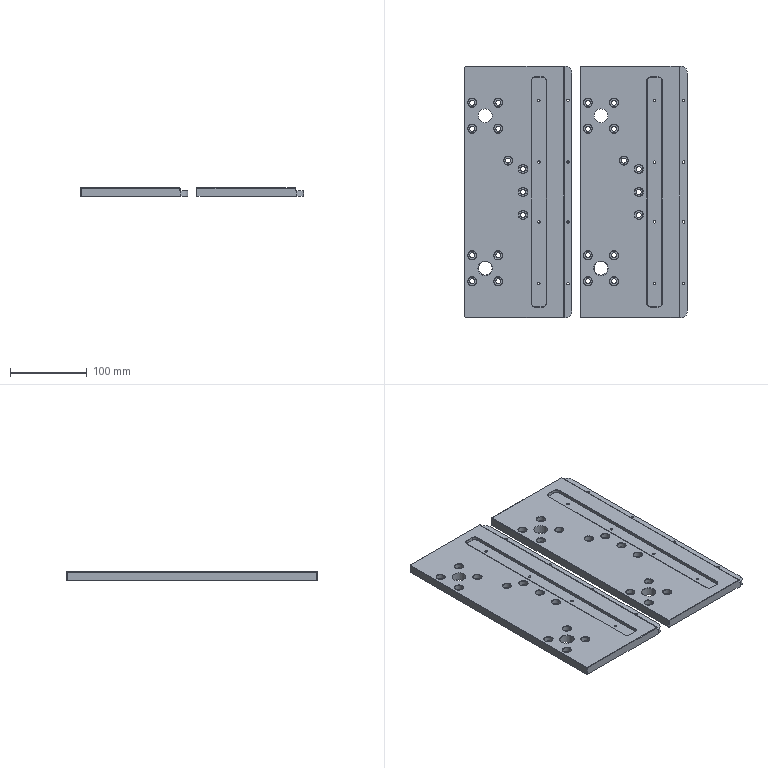CAM job | NX | 3-axis milling, drilling | part box 291 x 328 x 11 mm | stock box 296 x 333 x 12 mm
Tools:
number,name,description,diameter,corner_radius,flute_length,length,flutes
6,D6,平底铣刀-粗,6.0,0.0,25.0,75.0,2
9,D10,平底铣刀-粗,10.0,0.0,35.0,75.0,2
11,D2-J,平底铣刀-精,2.0,0.0,50.0,75.0,2
7,D6-J,平底铣刀-精,6.0,0.0,25.0,75.0,2
19,D6R0.5,圆鼻刀-粗,6.0,0.5,50.0,75.0,2
1,D80R0.8飞刀,圆鼻刀-粗,80.0,0.8,50.0,75.0,2
1,D80R0.8飞刀-J,圆鼻刀-精,80.0,0.8,50.0,75.0,2
2,D6倒角刀,倒角刀,6.0,0.0,3.0,25.0,2
13,ZT3.3,钻头,3.3,0.0,35.0,50.0,2
17,ZT6.5,钻头,6.5,0.0,35.0,50.0,2
18,ZT10,钻头,10.0,0.0,35.0,50.0,2
Operations:
program,operation,operation_type,tool,method,geometry_group,spindle_rpm,surface_speed,feed_per_tooth,feed_cut,feed_plunge,cut_length_mm,path_length_mm,cut_time_min,machine_time_min
A,底壁铣飞面开粗_COPY,VolumeBased25DMillingOperation,D80R0.8飞刀,分层开粗-切深K-步距G,W-A,5000.0,1256.637,0.3,3000.0,100.0,4565.572,5092.602,1.522,1.575
A,底壁铣飞面精光_COPY,VolumeBased25DMillingOperation,D80R0.8飞刀-J,侧刃精光-切深K-步距G,W-A,5000.0,1256.637,0.1,1000.0,100.0,2281.614,2317.614,2.282,2.285
A,打点,Operation,D6倒角刀,METHOD,W-A,3000.0,56.549,0.0333,200.0,0.0,110.0,1862.177,0.55,0.7252
A,打孔,Operation,ZT3.3,METHOD,W-A,3500.0,35.186,0.0143,100.0,0.0,184.0,1318.547,1.84,1.954
A,打孔_2,Operation,ZT6.5,METHOD,W-A,2500.0,51.051,0.03,150.0,0.0,276.0,1520.288,1.84,1.964
A,打孔_3,Operation,ZT10,METHOD,W-A,2000.0,62.832,0.03,120.0,0.0,46.0,636.009,0.3833,0.4423
A,台阶粗_2,CavityMilling,D10,METHOD,W-A,6000.0,188.0,0.25,3500.0,100.0,17169.813,18285.104,4.946,5.057
A,底壁粗_1,VolumeBased25DMillingOperation,D6,METHOD,W-A,6000.0,113.0,0.2083,3500.0,100.0,21552.928,22347.046,6.158,6.237
A,孔粗_1,CylinderMilling,D6,METHOD,W-A,6000.0,113.097,0.1667,2000.0,100.0,5829.376,7889.584,2.915,3.121
A,孔粗D6_3,CylinderMilling,D6,METHOD,W-A,6000.0,157.0,0.25,2500.0,90.0,3185.138,3436.738,1.275,1.3
A,孔粗D6_4,CylinderMilling,D6,METHOD,W-A,6000.0,157.0,0.25,2500.0,90.0,3263.684,3514.284,1.306,1.331
A,外形粗_2,VolumeBased25DMillingOperation,D10,METHOD,W-A,6000.0,188.0,0.25,4000.0,80.0,44123.768,44372.769,11.031,11.056
A,底精_1,VolumeBased25DMillingOperation,D6-J,METHOD,W-A,6000.0,113.0,0.2083,1200.0,100.0,2644.01,2959.71,2.203,2.235
A,底精_2,VolumeBased25DMillingOperation,D6-J,METHOD,W-A,6000.0,113.0,0.2083,1200.0,100.0,2478.352,2739.494,2.065,2.091
A,底侧精_3,VolumeBased25DMillingOperation,D6-J,METHOD,W-A,6000.0,113.0,0.2083,1200.0,100.0,678.37,1140.891,0.5653,0.6116
A,底侧精_4,VolumeBased25DMillingOperation,D6-J,METHOD,W-A,6000.0,113.0,0.2083,1200.0,100.0,1231.444,1488.125,1.026,1.052
A,孔侧_1,CylinderMilling,D6-J,METHOD,W-A,6000.0,113.097,0.0667,800.0,100.0,520.602,2756.011,0.6508,0.8743
A,孔侧E6_3,CylinderMilling,D6-J,METHOD,W-A,6000.0,157.0,0.2,800.0,90.0,158.413,432.812,0.1984,0.2258
A,孔侧E6_4,CylinderMilling,D6-J,METHOD,W-A,6000.0,157.0,0.2,800.0,90.0,158.413,432.802,0.1984,0.2258
A,底壁铣螺旋精光-中_COPY,VolumeBased25DMillingOperation,D2-J,螺旋精光-切深K-步距G,W-A,8000.0,50.264,0.0375,600.0,100.0,5018.468,7290.517,8.364,8.591
A,底壁铣螺旋精光-中_COPY_COPY,VolumeBased25DMillingOperation,D2-J,螺旋精光-切深K-步距G,W-A,8000.0,50.264,0.0375,600.0,100.0,1419.519,3169.978,2.366,2.541
A,等高精光往复爬面_COPY,ZLevelMilling,D6R0.5,等高爬面-切深K-步距G,W-A,7000.0,131.947,0.2857,4000.0,100.0,17678.729,17877.333,4.42,4.439
A,仅选体,SurfaceContour,D6倒角刀,METHOD,W-A,6000.0,113.0,0.125,1200.0,100.0,823.033,1560.856,0.6859,0.7596
A,钻倒角_1,Operation,D6倒角刀,METHOD,W-A,5000.0,94.248,0.015,150.0,0.0,82.4,1154.723,0.5493,0.6566
A,铣倒角_1,PlanarMilling,D6倒角刀,METHOD,W-A,6000.0,113.097,0.05,600.0,100.0,803.968,2780.644,1.34,1.538
A,外形半精_2,VolumeBased25DMillingOperation,D6-J,METHOD,W-A,6000.0,113.0,0.0833,1000.0,100.0,1901.737,2172.476,1.902,1.929
A,外形精_2,VolumeBased25DMillingOperation,D6-J,METHOD,W-A,6000.0,113.0,0.0833,1000.0,100.0,1901.337,2173.278,1.901,1.929